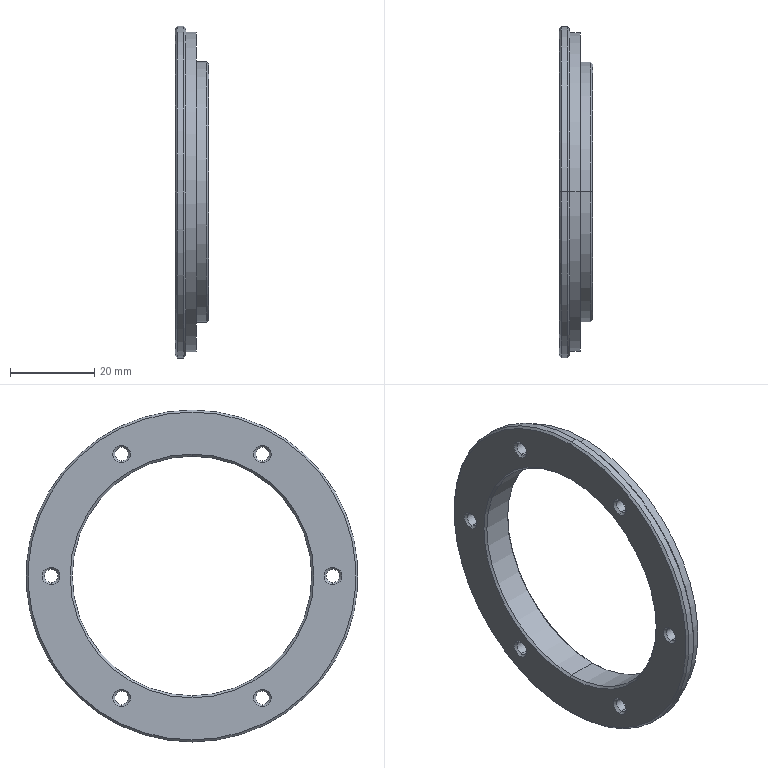Part | SolidWorks | features BaseBody 1, Chamfer 1, DelFace 1, MoveFace 1 | 1 solid | 58 faces | box 8 x 79 x 79 mm | volume 11850 mm3 | cone 34 | cylinder 20 | plane 4 | commonest cylinder face diameters 3.2 x12 57 x2 62 x2 76 x2 79 x2